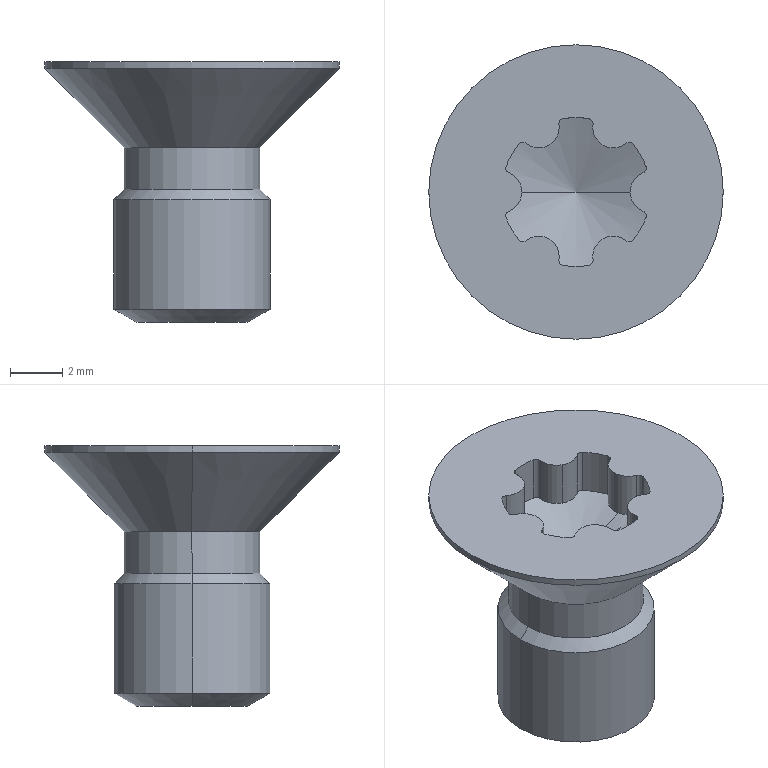Part | SolidWorks | features BaseBody 1 | 1 solid | 60 faces | box 11.3 x 11.3 x 10 mm | volume 323.209 mm3 | cylinder 44 | cone 8 | plane 8 | commonest cylinder face diameters 0.4 x20 1.57 x12 5.72 x6 5.196 x2 6 x2 11.3 x2